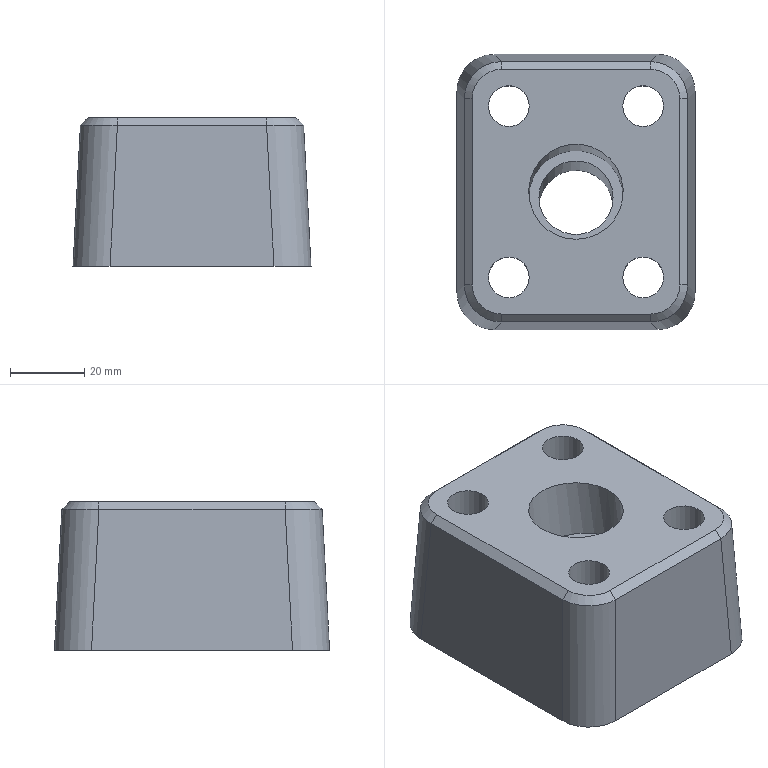Part | STEP file | solid 118 | 1 solid | 33 faces | box 64.193 x 74.193 x 40 mm | volume 137435 mm3 | plane 15 | cylinder 14 | spline 4 | commonest cylinder face diameters 20 x5 11 x4 18 x4 25.5 x1